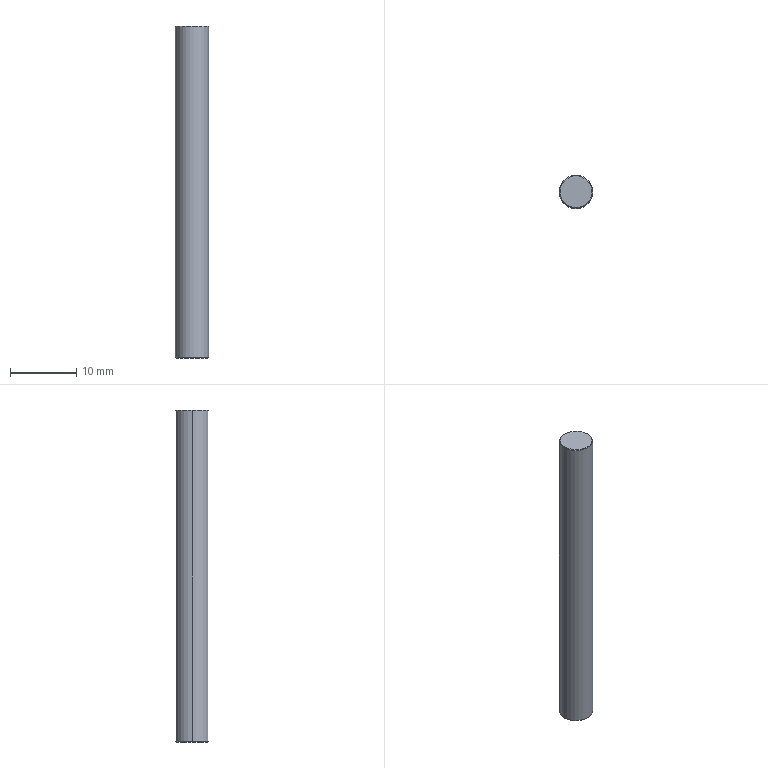Part | SolidWorks | features Chamfer 1, Extrusion 1 | 1 solid | 8 faces | box 5 x 5 x 50 mm | volume 981.593 mm3 | cone 4 | cylinder 2 | plane 2 | commonest cylinder face diameters 5 x2
STEP:
#1=CARTESIAN_POINT('',(-2.4,0.,-25.));
#2=VERTEX_POINT('',#1);
#3=CARTESIAN_POINT('',(2.4,0.,-25.));
#4=VERTEX_POINT('',#3);
#5=CARTESIAN_POINT('',(0.,0.,-25.));
#6=DIRECTION('',(0.,0.,-1.));
#7=DIRECTION('',(1.,0.,0.));
#8=AXIS2_PLACEMENT_3D('',#5,#6,#7);
#9=CIRCLE('',#8,2.4);
#10=EDGE_CURVE('',#2,#4,#9,.T.);
#11=ORIENTED_EDGE('',*,*,#10,.F.);
#12=CARTESIAN_POINT('',(-2.5,0.,-24.9));
#13=VERTEX_POINT('',#12);
#14=CARTESIAN_POINT('',(-2.5,0.,-24.9));
#15=DIRECTION('',(-0.7071,0.,0.7071));
#16=VECTOR('',#15,1000.);
#17=LINE('',#14,#16);
#18=EDGE_CURVE('',#2,#13,#17,.T.);
#19=ORIENTED_EDGE('',*,*,#18,.T.);
#20=CARTESIAN_POINT('',(2.5,0.,-24.9));
#21=VERTEX_POINT('',#20);
#22=CARTESIAN_POINT('',(0.,0.,-24.9));
#23=DIRECTION('',(0.,0.,1.));
#24=DIRECTION('',(1.,0.,0.));
#25=AXIS2_PLACEMENT_3D('',#22,#23,#24);
#26=CIRCLE('',#25,2.5);
#27=EDGE_CURVE('',#21,#13,#26,.T.);
#28=ORIENTED_EDGE('',*,*,#27,.F.);
#29=CARTESIAN_POINT('',(2.5,0.,-24.9));
#30=DIRECTION('',(0.7071,0.,0.7071));
#31=VECTOR('',#30,1000.);
#32=LINE('',#29,#31);
#33=EDGE_CURVE('',#4,#21,#32,.T.);
#34=ORIENTED_EDGE('',*,*,#33,.F.);
#35=EDGE_LOOP('',(#11,#19,#28,#34));
#36=FACE_OUTER_BOUND('',#35,.T.);
#37=CARTESIAN_POINT('',(0.,0.,-24.9));
#38=DIRECTION('',(0.,0.,1.));
#39=DIRECTION('',(1.,0.,0.));
#40=AXIS2_PLACEMENT_3D('',#37,#38,#39);
#41=CONICAL_SURFACE('',#40,2.5,0.7854);
#42=ADVANCED_FACE('',(#36),#41,.T.);
#43=CARTESIAN_POINT('',(2.4,0.,25.));
#44=VERTEX_POINT('',#43);
#45=CARTESIAN_POINT('',(-2.4,0.,25.));
#46=VERTEX_POINT('',#45);
#47=CARTESIAN_POINT('',(0.,0.,25.));
#48=DIRECTION('',(0.,0.,1.));
#49=DIRECTION('',(1.,0.,0.));
#50=AXIS2_PLACEMENT_3D('',#47,#48,#49);
#51=CIRCLE('',#50,2.4);
#52=EDGE_CURVE('',#44,#46,#51,.T.);
#53=ORIENTED_EDGE('',*,*,#52,.F.);
#54=CARTESIAN_POINT('',(2.5,0.,24.9));
#55=VERTEX_POINT('',#54);
#56=CARTESIAN_POINT('',(2.4,0.,25.));
#57=DIRECTION('',(0.7071,0.,-0.7071));
#58=VECTOR('',#57,1000.);
#59=LINE('',#56,#58);
#60=EDGE_CURVE('',#44,#55,#59,.T.);
#61=ORIENTED_EDGE('',*,*,#60,.T.);
#62=CARTESIAN_POINT('',(-2.5,0.,24.9));
#63=VERTEX_POINT('',#62);
#64=CARTESIAN_POINT('',(0.,0.,24.9));
#65=DIRECTION('',(0.,0.,-1.));
#66=DIRECTION('',(1.,0.,0.));
#67=AXIS2_PLACEMENT_3D('',#64,#65,#66);
#68=CIRCLE('',#67,2.5);
#69=EDGE_CURVE('',#63,#55,#68,.T.);
#70=ORIENTED_EDGE('',*,*,#69,.F.);
#71=CARTESIAN_POINT('',(-2.4,0.,25.));
#72=DIRECTION('',(-0.7071,0.,-0.7071));
#73=VECTOR('',#72,1000.);
#74=LINE('',#71,#73);
#75=EDGE_CURVE('',#46,#63,#74,.T.);
#76=ORIENTED_EDGE('',*,*,#75,.F.);
#77=EDGE_LOOP('',(#53,#61,#70,#76));
#78=FACE_OUTER_BOUND('',#77,.T.);
#79=CARTESIAN_POINT('',(0.,0.,25.));
#80=DIRECTION('',(0.,0.,-1.));
#81=DIRECTION('',(-1.,0.,0.));
#82=AXIS2_PLACEMENT_3D('',#79,#80,#81);
#83=CONICAL_SURFACE('',#82,2.4,0.7854);
#84=ADVANCED_FACE('',(#78),#83,.T.);
#85=ORIENTED_EDGE('',*,*,#69,.T.);
#86=CARTESIAN_POINT('',(2.5,0.,25.));
#87=DIRECTION('',(0.,0.,-1.));
#88=VECTOR('',#87,1000.);
#89=LINE('',#86,#88);
#90=EDGE_CURVE('',#55,#21,#89,.T.);
#91=ORIENTED_EDGE('',*,*,#90,.T.);
#92=ORIENTED_EDGE('',*,*,#27,.T.);
#93=CARTESIAN_POINT('',(-2.5,0.,25.));
#94=DIRECTION('',(0.,0.,-1.));
#95=VECTOR('',#94,1000.);
#96=LINE('',#93,#95);
#97=EDGE_CURVE('',#63,#13,#96,.T.);
#98=ORIENTED_EDGE('',*,*,#97,.F.);
#99=EDGE_LOOP('',(#85,#91,#92,#98));
#100=FACE_OUTER_BOUND('',#99,.T.);
#101=CARTESIAN_POINT('',(0.,0.,25.));
#102=DIRECTION('',(0.,0.,-1.));
#103=DIRECTION('',(-1.,0.,0.));
#104=AXIS2_PLACEMENT_3D('',#101,#102,#103);
#105=CYLINDRICAL_SURFACE('',#104,2.5);
#106=ADVANCED_FACE('',(#100),#105,.T.);
#107=ORIENTED_EDGE('',*,*,#90,.F.);
#108=CARTESIAN_POINT('',(0.,0.,24.9));
#109=DIRECTION('',(0.,0.,-1.));
#110=DIRECTION('',(1.,0.,0.));
#111=AXIS2_PLACEMENT_3D('',#108,#109,#110);
#112=CIRCLE('',#111,2.5);
#113=EDGE_CURVE('',#55,#63,#112,.T.);
#114=ORIENTED_EDGE('',*,*,#113,.T.);
#115=ORIENTED_EDGE('',*,*,#97,.T.);
#116=CARTESIAN_POINT('',(0.,0.,-24.9));
#117=DIRECTION('',(0.,0.,1.));
#118=DIRECTION('',(1.,0.,0.));
#119=AXIS2_PLACEMENT_3D('',#116,#117,#118);
#120=CIRCLE('',#119,2.5);
#121=EDGE_CURVE('',#13,#21,#120,.T.);
#122=ORIENTED_EDGE('',*,*,#121,.T.);
#123=EDGE_LOOP('',(#107,#114,#115,#122));
#124=FACE_OUTER_BOUND('',#123,.T.);
#125=CARTESIAN_POINT('',(0.,0.,25.));
#126=DIRECTION('',(0.,0.,-1.));
#127=DIRECTION('',(-1.,0.,0.));
#128=AXIS2_PLACEMENT_3D('',#125,#126,#127);
#129=CYLINDRICAL_SURFACE('',#128,2.5);
#130=ADVANCED_FACE('',(#124),#129,.T.);
#131=CARTESIAN_POINT('',(0.,0.,25.));
#132=DIRECTION('',(0.,0.,1.));
#133=DIRECTION('',(1.,0.,0.));
#134=AXIS2_PLACEMENT_3D('',#131,#132,#133);
#135=CIRCLE('',#134,2.4);
#136=EDGE_CURVE('',#46,#44,#135,.T.);
#137=ORIENTED_EDGE('',*,*,#136,.T.);
#138=ORIENTED_EDGE('',*,*,#52,.T.);
#139=EDGE_LOOP('',(#137,#138));
#140=FACE_OUTER_BOUND('',#139,.T.);
#141=CARTESIAN_POINT('',(0.,0.,25.));
#142=DIRECTION('',(0.,0.,1.));
#143=DIRECTION('',(1.,0.,0.));
#144=AXIS2_PLACEMENT_3D('',#141,#142,#143);
#145=PLANE('',#144);
#146=ADVANCED_FACE('',(#140),#145,.T.);
#147=CARTESIAN_POINT('',(0.,0.,-25.));
#148=DIRECTION('',(0.,0.,-1.));
#149=DIRECTION('',(1.,0.,0.));
#150=AXIS2_PLACEMENT_3D('',#147,#148,#149);
#151=CIRCLE('',#150,2.4);
#152=EDGE_CURVE('',#4,#2,#151,.T.);
#153=ORIENTED_EDGE('',*,*,#152,.T.);
#154=ORIENTED_EDGE('',*,*,#10,.T.);
#155=EDGE_LOOP('',(#153,#154));
#156=FACE_OUTER_BOUND('',#155,.T.);
#157=CARTESIAN_POINT('',(0.,0.,-25.));
#158=DIRECTION('',(0.,0.,1.));
#159=DIRECTION('',(1.,0.,0.));
#160=AXIS2_PLACEMENT_3D('',#157,#158,#159);
#161=PLANE('',#160);
#162=ADVANCED_FACE('',(#156),#161,.F.);
#163=ORIENTED_EDGE('',*,*,#60,.F.);
#164=ORIENTED_EDGE('',*,*,#136,.F.);
#165=ORIENTED_EDGE('',*,*,#75,.T.);
#166=ORIENTED_EDGE('',*,*,#113,.F.);
#167=EDGE_LOOP('',(#163,#164,#165,#166));
#168=FACE_OUTER_BOUND('',#167,.T.);
#169=CARTESIAN_POINT('',(0.,0.,25.));
#170=DIRECTION('',(0.,0.,-1.));
#171=DIRECTION('',(-1.,0.,0.));
#172=AXIS2_PLACEMENT_3D('',#169,#170,#171);
#173=CONICAL_SURFACE('',#172,2.4,0.7854);
#174=ADVANCED_FACE('',(#168),#173,.T.);
#175=ORIENTED_EDGE('',*,*,#18,.F.);
#176=ORIENTED_EDGE('',*,*,#152,.F.);
#177=ORIENTED_EDGE('',*,*,#33,.T.);
#178=ORIENTED_EDGE('',*,*,#121,.F.);
#179=EDGE_LOOP('',(#175,#176,#177,#178));
#180=FACE_OUTER_BOUND('',#179,.T.);
#181=CARTESIAN_POINT('',(0.,0.,-24.9));
#182=DIRECTION('',(0.,0.,1.));
#183=DIRECTION('',(1.,0.,0.));
#184=AXIS2_PLACEMENT_3D('',#181,#182,#183);
#185=CONICAL_SURFACE('',#184,2.5,0.7854);
#186=ADVANCED_FACE('',(#180),#185,.T.);
#187=CLOSED_SHELL('',(#42,#84,#106,#130,#146,#162,#174,#186));
#188=MANIFOLD_SOLID_BREP('',#187);
#189=CARTESIAN_POINT('',(0.,0.,0.));
#190=DIRECTION('',(0.,0.,1.));
#191=DIRECTION('',(1.,0.,0.));
#192=AXIS2_PLACEMENT_3D('',#189,#190,#191);
#193=(LENGTH_UNIT()NAMED_UNIT(*)SI_UNIT(.MILLI.,.METRE.));
#194=UNCERTAINTY_MEASURE_WITH_UNIT(LENGTH_MEASURE(0.00001),#193,'','');
#195=(NAMED_UNIT(*)PLANE_ANGLE_UNIT()SI_UNIT($,.RADIAN.));
#196=(NAMED_UNIT(*)SI_UNIT($,.STERADIAN.)SOLID_ANGLE_UNIT());
#197=(GEOMETRIC_REPRESENTATION_CONTEXT(3)GLOBAL_UNCERTAINTY_ASSIGNED_CONTEXT((#194))GLOBAL_UNIT_ASSIGNED_CONTEXT((#193,#195,#196))REPRESENTATION_CONTEXT('',''));
#198=ADVANCED_BREP_SHAPE_REPRESENTATION('',(#188,#192),#197);